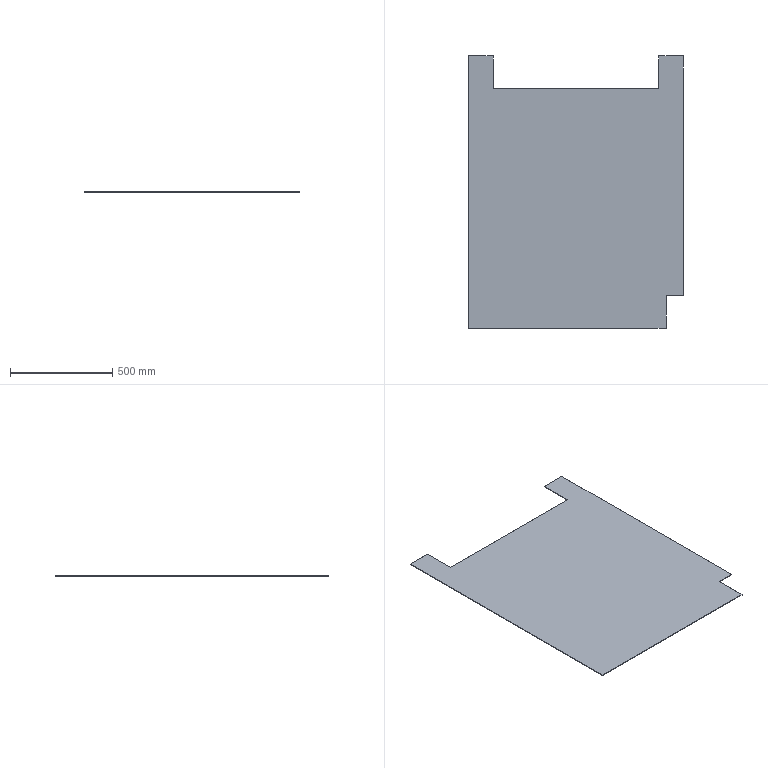Part | STEP file | Electrical cabinet stair checkered plate | 1 solid | 12 faces | box 1050 x 1330 x 3 mm | volume 3760665 mm3 | plane 12
STEP:
#1=CARTESIAN_POINT('',(0.,0.,0.));
#2=DIRECTION('',(0.,0.,1.));
#3=DIRECTION('',(1.,0.,0.));
#4=AXIS2_PLACEMENT_3D('',#1,#2,#3);
#5=CARTESIAN_POINT('',(1215.,107.,0.));
#6=VERTEX_POINT('',#5);
#7=CARTESIAN_POINT('',(1300.,107.,0.));
#8=VERTEX_POINT('',#7);
#9=CARTESIAN_POINT('',(1215.,107.,0.));
#10=DIRECTION('',(1.,0.,0.));
#11=VECTOR('',#10,1.);
#12=LINE('',#9,#11);
#13=CARTESIAN_POINT('',(1215.,107.,3.));
#14=DIRECTION('',(0.,1.,0.));
#15=DIRECTION('',(0.,0.,1.));
#16=AXIS2_PLACEMENT_3D('',#13,#14,#15);
#17=PLANE('',#16);
#18=CARTESIAN_POINT('',(-3.,0.));
#19=DIRECTION('',(0.,1.));
#20=VECTOR('',#19,1.);
#21=LINE('',#18,#20);
#22=(GEOMETRIC_REPRESENTATION_CONTEXT(2)PARAMETRIC_REPRESENTATION_CONTEXT()REPRESENTATION_CONTEXT('',''));
#23=DEFINITIONAL_REPRESENTATION('',(#21),#22);
#24=PCURVE('',#17,#23);
#25=CARTESIAN_POINT('',(0.,0.,0.));
#26=DIRECTION('',(0.,0.,1.));
#27=DIRECTION('',(1.,0.,0.));
#28=AXIS2_PLACEMENT_3D('',#25,#26,#27);
#29=PLANE('',#28);
#30=CARTESIAN_POINT('',(1215.,107.));
#31=DIRECTION('',(1.,0.));
#32=VECTOR('',#31,1.);
#33=LINE('',#30,#32);
#34=(GEOMETRIC_REPRESENTATION_CONTEXT(2)PARAMETRIC_REPRESENTATION_CONTEXT()REPRESENTATION_CONTEXT('',''));
#35=DEFINITIONAL_REPRESENTATION('',(#33),#34);
#36=PCURVE('',#29,#35);
#37=SURFACE_CURVE('',#12,(#24,#36),.PCURVE_S1.);
#38=EDGE_CURVE('',#6,#8,#37,.T.);
#39=ORIENTED_EDGE('',*,*,#38,.T.);
#40=CARTESIAN_POINT('',(1300.,107.,3.));
#41=VERTEX_POINT('',#40);
#42=CARTESIAN_POINT('',(1300.,107.,3.));
#43=DIRECTION('',(0.,0.,-1.));
#44=VECTOR('',#43,1.);
#45=LINE('',#42,#44);
#46=CARTESIAN_POINT('',(0.,85.));
#47=DIRECTION('',(-1.,0.));
#48=VECTOR('',#47,1.);
#49=LINE('',#46,#48);
#50=(GEOMETRIC_REPRESENTATION_CONTEXT(2)PARAMETRIC_REPRESENTATION_CONTEXT()REPRESENTATION_CONTEXT('',''));
#51=DEFINITIONAL_REPRESENTATION('',(#49),#50);
#52=PCURVE('',#17,#51);
#53=CARTESIAN_POINT('',(1300.,107.,3.));
#54=DIRECTION('',(-1.,0.,0.));
#55=DIRECTION('',(0.,-1.,0.));
#56=AXIS2_PLACEMENT_3D('',#53,#54,#55);
#57=PLANE('',#56);
#58=CARTESIAN_POINT('',(0.,0.));
#59=DIRECTION('',(0.,-1.));
#60=VECTOR('',#59,1.);
#61=LINE('',#58,#60);
#62=(GEOMETRIC_REPRESENTATION_CONTEXT(2)PARAMETRIC_REPRESENTATION_CONTEXT()REPRESENTATION_CONTEXT('',''));
#63=DEFINITIONAL_REPRESENTATION('',(#61),#62);
#64=PCURVE('',#57,#63);
#65=SURFACE_CURVE('',#45,(#52,#64),.PCURVE_S1.);
#66=EDGE_CURVE('',#41,#8,#65,.T.);
#67=ORIENTED_EDGE('',*,*,#66,.F.);
#68=CARTESIAN_POINT('',(1215.,107.,3.));
#69=VERTEX_POINT('',#68);
#70=CARTESIAN_POINT('',(1215.,107.,3.));
#71=DIRECTION('',(1.,0.,0.));
#72=VECTOR('',#71,1.);
#73=LINE('',#70,#72);
#74=CARTESIAN_POINT('',(0.,0.));
#75=DIRECTION('',(0.,1.));
#76=VECTOR('',#75,1.);
#77=LINE('',#74,#76);
#78=(GEOMETRIC_REPRESENTATION_CONTEXT(2)PARAMETRIC_REPRESENTATION_CONTEXT()REPRESENTATION_CONTEXT('',''));
#79=DEFINITIONAL_REPRESENTATION('',(#77),#78);
#80=PCURVE('',#17,#79);
#81=CARTESIAN_POINT('',(0.,0.,3.));
#82=DIRECTION('',(0.,0.,1.));
#83=DIRECTION('',(1.,0.,0.));
#84=AXIS2_PLACEMENT_3D('',#81,#82,#83);
#85=PLANE('',#84);
#86=CARTESIAN_POINT('',(1215.,107.));
#87=DIRECTION('',(1.,0.));
#88=VECTOR('',#87,1.);
#89=LINE('',#86,#88);
#90=(GEOMETRIC_REPRESENTATION_CONTEXT(2)PARAMETRIC_REPRESENTATION_CONTEXT()REPRESENTATION_CONTEXT('',''));
#91=DEFINITIONAL_REPRESENTATION('',(#89),#90);
#92=PCURVE('',#85,#91);
#93=SURFACE_CURVE('',#73,(#80,#92),.PCURVE_S1.);
#94=EDGE_CURVE('',#69,#41,#93,.T.);
#95=ORIENTED_EDGE('',*,*,#94,.F.);
#96=CARTESIAN_POINT('',(1215.,107.,3.));
#97=DIRECTION('',(0.,0.,-1.));
#98=VECTOR('',#97,1.);
#99=LINE('',#96,#98);
#100=CARTESIAN_POINT('',(0.,0.));
#101=DIRECTION('',(-1.,0.));
#102=VECTOR('',#101,1.);
#103=LINE('',#100,#102);
#104=(GEOMETRIC_REPRESENTATION_CONTEXT(2)PARAMETRIC_REPRESENTATION_CONTEXT()REPRESENTATION_CONTEXT('',''));
#105=DEFINITIONAL_REPRESENTATION('',(#103),#104);
#106=PCURVE('',#17,#105);
#107=CARTESIAN_POINT('',(1215.,-50.,3.));
#108=DIRECTION('',(-1.,0.,0.));
#109=DIRECTION('',(0.,0.,1.));
#110=AXIS2_PLACEMENT_3D('',#107,#108,#109);
#111=PLANE('',#110);
#112=CARTESIAN_POINT('',(0.,157.));
#113=DIRECTION('',(-1.,0.));
#114=VECTOR('',#113,1.);
#115=LINE('',#112,#114);
#116=(GEOMETRIC_REPRESENTATION_CONTEXT(2)PARAMETRIC_REPRESENTATION_CONTEXT()REPRESENTATION_CONTEXT('',''));
#117=DEFINITIONAL_REPRESENTATION('',(#115),#116);
#118=PCURVE('',#111,#117);
#119=SURFACE_CURVE('',#99,(#106,#118),.PCURVE_S1.);
#120=EDGE_CURVE('',#69,#6,#119,.T.);
#121=ORIENTED_EDGE('',*,*,#120,.T.);
#122=EDGE_LOOP('',(#39,#67,#95,#121));
#123=FACE_BOUND('',#122,.T.);
#124=ADVANCED_FACE('',(#123),#17,.F.);
#125=CARTESIAN_POINT('',(1300.,1280.,0.));
#126=VERTEX_POINT('',#125);
#127=CARTESIAN_POINT('',(1300.,107.,0.));
#128=DIRECTION('',(0.,1.,0.));
#129=VECTOR('',#128,1.);
#130=LINE('',#127,#129);
#131=CARTESIAN_POINT('',(0.,-3.));
#132=DIRECTION('',(-1.,0.));
#133=VECTOR('',#132,1.);
#134=LINE('',#131,#133);
#135=(GEOMETRIC_REPRESENTATION_CONTEXT(2)PARAMETRIC_REPRESENTATION_CONTEXT()REPRESENTATION_CONTEXT('',''));
#136=DEFINITIONAL_REPRESENTATION('',(#134),#135);
#137=PCURVE('',#57,#136);
#138=CARTESIAN_POINT('',(1300.,107.));
#139=DIRECTION('',(0.,1.));
#140=VECTOR('',#139,1.);
#141=LINE('',#138,#140);
#142=(GEOMETRIC_REPRESENTATION_CONTEXT(2)PARAMETRIC_REPRESENTATION_CONTEXT()REPRESENTATION_CONTEXT('',''));
#143=DEFINITIONAL_REPRESENTATION('',(#141),#142);
#144=PCURVE('',#29,#143);
#145=SURFACE_CURVE('',#130,(#137,#144),.PCURVE_S1.);
#146=EDGE_CURVE('',#8,#126,#145,.T.);
#147=ORIENTED_EDGE('',*,*,#146,.T.);
#148=CARTESIAN_POINT('',(1300.,1280.,3.));
#149=VERTEX_POINT('',#148);
#150=CARTESIAN_POINT('',(1300.,1280.,3.));
#151=DIRECTION('',(0.,0.,-1.));
#152=VECTOR('',#151,1.);
#153=LINE('',#150,#152);
#154=CARTESIAN_POINT('',(-1173.,0.));
#155=DIRECTION('',(0.,-1.));
#156=VECTOR('',#155,1.);
#157=LINE('',#154,#156);
#158=(GEOMETRIC_REPRESENTATION_CONTEXT(2)PARAMETRIC_REPRESENTATION_CONTEXT()REPRESENTATION_CONTEXT('',''));
#159=DEFINITIONAL_REPRESENTATION('',(#157),#158);
#160=PCURVE('',#57,#159);
#161=CARTESIAN_POINT('',(1300.,1280.,3.));
#162=DIRECTION('',(0.,-1.,0.));
#163=DIRECTION('',(0.,0.,-1.));
#164=AXIS2_PLACEMENT_3D('',#161,#162,#163);
#165=PLANE('',#164);
#166=CARTESIAN_POINT('',(0.,0.));
#167=DIRECTION('',(1.,0.));
#168=VECTOR('',#167,1.);
#169=LINE('',#166,#168);
#170=(GEOMETRIC_REPRESENTATION_CONTEXT(2)PARAMETRIC_REPRESENTATION_CONTEXT()REPRESENTATION_CONTEXT('',''));
#171=DEFINITIONAL_REPRESENTATION('',(#169),#170);
#172=PCURVE('',#165,#171);
#173=SURFACE_CURVE('',#153,(#160,#172),.PCURVE_S1.);
#174=EDGE_CURVE('',#149,#126,#173,.T.);
#175=ORIENTED_EDGE('',*,*,#174,.F.);
#176=CARTESIAN_POINT('',(1300.,107.,3.));
#177=DIRECTION('',(0.,1.,0.));
#178=VECTOR('',#177,1.);
#179=LINE('',#176,#178);
#180=CARTESIAN_POINT('',(0.,0.));
#181=DIRECTION('',(-1.,0.));
#182=VECTOR('',#181,1.);
#183=LINE('',#180,#182);
#184=(GEOMETRIC_REPRESENTATION_CONTEXT(2)PARAMETRIC_REPRESENTATION_CONTEXT()REPRESENTATION_CONTEXT('',''));
#185=DEFINITIONAL_REPRESENTATION('',(#183),#184);
#186=PCURVE('',#57,#185);
#187=CARTESIAN_POINT('',(1300.,107.));
#188=DIRECTION('',(0.,1.));
#189=VECTOR('',#188,1.);
#190=LINE('',#187,#189);
#191=(GEOMETRIC_REPRESENTATION_CONTEXT(2)PARAMETRIC_REPRESENTATION_CONTEXT()REPRESENTATION_CONTEXT('',''));
#192=DEFINITIONAL_REPRESENTATION('',(#190),#191);
#193=PCURVE('',#85,#192);
#194=SURFACE_CURVE('',#179,(#186,#193),.PCURVE_S1.);
#195=EDGE_CURVE('',#41,#149,#194,.T.);
#196=ORIENTED_EDGE('',*,*,#195,.F.);
#197=ORIENTED_EDGE('',*,*,#66,.T.);
#198=EDGE_LOOP('',(#147,#175,#196,#197));
#199=FACE_BOUND('',#198,.T.);
#200=ADVANCED_FACE('',(#199),#57,.F.);
#201=CARTESIAN_POINT('',(1180.,1280.,0.));
#202=VERTEX_POINT('',#201);
#203=CARTESIAN_POINT('',(1300.,1280.,0.));
#204=DIRECTION('',(-1.,0.,0.));
#205=VECTOR('',#204,1.);
#206=LINE('',#203,#205);
#207=CARTESIAN_POINT('',(3.,0.));
#208=DIRECTION('',(0.,-1.));
#209=VECTOR('',#208,1.);
#210=LINE('',#207,#209);
#211=(GEOMETRIC_REPRESENTATION_CONTEXT(2)PARAMETRIC_REPRESENTATION_CONTEXT()REPRESENTATION_CONTEXT('',''));
#212=DEFINITIONAL_REPRESENTATION('',(#210),#211);
#213=PCURVE('',#165,#212);
#214=CARTESIAN_POINT('',(1300.,1280.));
#215=DIRECTION('',(-1.,0.));
#216=VECTOR('',#215,1.);
#217=LINE('',#214,#216);
#218=(GEOMETRIC_REPRESENTATION_CONTEXT(2)PARAMETRIC_REPRESENTATION_CONTEXT()REPRESENTATION_CONTEXT('',''));
#219=DEFINITIONAL_REPRESENTATION('',(#217),#218);
#220=PCURVE('',#29,#219);
#221=SURFACE_CURVE('',#206,(#213,#220),.PCURVE_S1.);
#222=EDGE_CURVE('',#126,#202,#221,.T.);
#223=ORIENTED_EDGE('',*,*,#222,.T.);
#224=CARTESIAN_POINT('',(1180.,1280.,3.));
#225=VERTEX_POINT('',#224);
#226=CARTESIAN_POINT('',(1180.,1280.,3.));
#227=DIRECTION('',(0.,0.,-1.));
#228=VECTOR('',#227,1.);
#229=LINE('',#226,#228);
#230=CARTESIAN_POINT('',(0.,-120.));
#231=DIRECTION('',(1.,0.));
#232=VECTOR('',#231,1.);
#233=LINE('',#230,#232);
#234=(GEOMETRIC_REPRESENTATION_CONTEXT(2)PARAMETRIC_REPRESENTATION_CONTEXT()REPRESENTATION_CONTEXT('',''));
#235=DEFINITIONAL_REPRESENTATION('',(#233),#234);
#236=PCURVE('',#165,#235);
#237=CARTESIAN_POINT('',(1180.,1120.,3.));
#238=DIRECTION('',(1.,0.,0.));
#239=DIRECTION('',(0.,0.,-1.));
#240=AXIS2_PLACEMENT_3D('',#237,#238,#239);
#241=PLANE('',#240);
#242=CARTESIAN_POINT('',(0.,160.));
#243=DIRECTION('',(1.,0.));
#244=VECTOR('',#243,1.);
#245=LINE('',#242,#244);
#246=(GEOMETRIC_REPRESENTATION_CONTEXT(2)PARAMETRIC_REPRESENTATION_CONTEXT()REPRESENTATION_CONTEXT('',''));
#247=DEFINITIONAL_REPRESENTATION('',(#245),#246);
#248=PCURVE('',#241,#247);
#249=SURFACE_CURVE('',#229,(#236,#248),.PCURVE_S1.);
#250=EDGE_CURVE('',#225,#202,#249,.T.);
#251=ORIENTED_EDGE('',*,*,#250,.F.);
#252=CARTESIAN_POINT('',(1300.,1280.,3.));
#253=DIRECTION('',(-1.,0.,0.));
#254=VECTOR('',#253,1.);
#255=LINE('',#252,#254);
#256=CARTESIAN_POINT('',(0.,0.));
#257=DIRECTION('',(0.,-1.));
#258=VECTOR('',#257,1.);
#259=LINE('',#256,#258);
#260=(GEOMETRIC_REPRESENTATION_CONTEXT(2)PARAMETRIC_REPRESENTATION_CONTEXT()REPRESENTATION_CONTEXT('',''));
#261=DEFINITIONAL_REPRESENTATION('',(#259),#260);
#262=PCURVE('',#165,#261);
#263=CARTESIAN_POINT('',(1300.,1280.));
#264=DIRECTION('',(-1.,0.));
#265=VECTOR('',#264,1.);
#266=LINE('',#263,#265);
#267=(GEOMETRIC_REPRESENTATION_CONTEXT(2)PARAMETRIC_REPRESENTATION_CONTEXT()REPRESENTATION_CONTEXT('',''));
#268=DEFINITIONAL_REPRESENTATION('',(#266),#267);
#269=PCURVE('',#85,#268);
#270=SURFACE_CURVE('',#255,(#262,#269),.PCURVE_S1.);
#271=EDGE_CURVE('',#149,#225,#270,.T.);
#272=ORIENTED_EDGE('',*,*,#271,.F.);
#273=ORIENTED_EDGE('',*,*,#174,.T.);
#274=EDGE_LOOP('',(#223,#251,#272,#273));
#275=FACE_BOUND('',#274,.T.);
#276=ADVANCED_FACE('',(#275),#165,.F.);
#277=CARTESIAN_POINT('',(1180.,1120.,0.));
#278=VERTEX_POINT('',#277);
#279=CARTESIAN_POINT('',(1180.,1120.,0.));
#280=DIRECTION('',(0.,-1.,0.));
#281=VECTOR('',#280,1.);
#282=LINE('',#279,#281);
#283=CARTESIAN_POINT('',(3.,0.));
#284=DIRECTION('',(0.,-1.));
#285=VECTOR('',#284,1.);
#286=LINE('',#283,#285);
#287=(GEOMETRIC_REPRESENTATION_CONTEXT(2)PARAMETRIC_REPRESENTATION_CONTEXT()REPRESENTATION_CONTEXT('',''));
#288=DEFINITIONAL_REPRESENTATION('',(#286),#287);
#289=PCURVE('',#241,#288);
#290=CARTESIAN_POINT('',(1180.,1120.));
#291=DIRECTION('',(0.,-1.));
#292=VECTOR('',#291,1.);
#293=LINE('',#290,#292);
#294=(GEOMETRIC_REPRESENTATION_CONTEXT(2)PARAMETRIC_REPRESENTATION_CONTEXT()REPRESENTATION_CONTEXT('',''));
#295=DEFINITIONAL_REPRESENTATION('',(#293),#294);
#296=PCURVE('',#29,#295);
#297=SURFACE_CURVE('',#282,(#289,#296),.PCURVE_S1.);
#298=EDGE_CURVE('',#202,#278,#297,.T.);
#299=ORIENTED_EDGE('',*,*,#298,.T.);
#300=CARTESIAN_POINT('',(1180.,1120.,3.));
#301=VERTEX_POINT('',#300);
#302=CARTESIAN_POINT('',(1180.,1120.,3.));
#303=DIRECTION('',(0.,0.,-1.));
#304=VECTOR('',#303,1.);
#305=LINE('',#302,#304);
#306=CARTESIAN_POINT('',(0.,0.));
#307=DIRECTION('',(1.,0.));
#308=VECTOR('',#307,1.);
#309=LINE('',#306,#308);
#310=(GEOMETRIC_REPRESENTATION_CONTEXT(2)PARAMETRIC_REPRESENTATION_CONTEXT()REPRESENTATION_CONTEXT('',''));
#311=DEFINITIONAL_REPRESENTATION('',(#309),#310);
#312=PCURVE('',#241,#311);
#313=CARTESIAN_POINT('',(370.,1120.,3.));
#314=DIRECTION('',(0.,-1.,0.));
#315=DIRECTION('',(0.,0.,-1.));
#316=AXIS2_PLACEMENT_3D('',#313,#314,#315);
#317=PLANE('',#316);
#318=CARTESIAN_POINT('',(0.,810.));
#319=DIRECTION('',(1.,0.));
#320=VECTOR('',#319,1.);
#321=LINE('',#318,#320);
#322=(GEOMETRIC_REPRESENTATION_CONTEXT(2)PARAMETRIC_REPRESENTATION_CONTEXT()REPRESENTATION_CONTEXT('',''));
#323=DEFINITIONAL_REPRESENTATION('',(#321),#322);
#324=PCURVE('',#317,#323);
#325=SURFACE_CURVE('',#305,(#312,#324),.PCURVE_S1.);
#326=EDGE_CURVE('',#301,#278,#325,.T.);
#327=ORIENTED_EDGE('',*,*,#326,.F.);
#328=CARTESIAN_POINT('',(1180.,1120.,3.));
#329=DIRECTION('',(0.,-1.,0.));
#330=VECTOR('',#329,1.);
#331=LINE('',#328,#330);
#332=CARTESIAN_POINT('',(0.,0.));
#333=DIRECTION('',(0.,-1.));
#334=VECTOR('',#333,1.);
#335=LINE('',#332,#334);
#336=(GEOMETRIC_REPRESENTATION_CONTEXT(2)PARAMETRIC_REPRESENTATION_CONTEXT()REPRESENTATION_CONTEXT('',''));
#337=DEFINITIONAL_REPRESENTATION('',(#335),#336);
#338=PCURVE('',#241,#337);
#339=CARTESIAN_POINT('',(1180.,1120.));
#340=DIRECTION('',(0.,-1.));
#341=VECTOR('',#340,1.);
#342=LINE('',#339,#341);
#343=(GEOMETRIC_REPRESENTATION_CONTEXT(2)PARAMETRIC_REPRESENTATION_CONTEXT()REPRESENTATION_CONTEXT('',''));
#344=DEFINITIONAL_REPRESENTATION('',(#342),#343);
#345=PCURVE('',#85,#344);
#346=SURFACE_CURVE('',#331,(#338,#345),.PCURVE_S1.);
#347=EDGE_CURVE('',#225,#301,#346,.T.);
#348=ORIENTED_EDGE('',*,*,#347,.F.);
#349=ORIENTED_EDGE('',*,*,#250,.T.);
#350=EDGE_LOOP('',(#299,#327,#348,#349));
#351=FACE_BOUND('',#350,.T.);
#352=ADVANCED_FACE('',(#351),#241,.F.);
#353=CARTESIAN_POINT('',(370.,1120.,0.));
#354=VERTEX_POINT('',#353);
#355=CARTESIAN_POINT('',(370.,1120.,0.));
#356=DIRECTION('',(-1.,0.,0.));
#357=VECTOR('',#356,1.);
#358=LINE('',#355,#357);
#359=CARTESIAN_POINT('',(3.,0.));
#360=DIRECTION('',(0.,-1.));
#361=VECTOR('',#360,1.);
#362=LINE('',#359,#361);
#363=(GEOMETRIC_REPRESENTATION_CONTEXT(2)PARAMETRIC_REPRESENTATION_CONTEXT()REPRESENTATION_CONTEXT('',''));
#364=DEFINITIONAL_REPRESENTATION('',(#362),#363);
#365=PCURVE('',#317,#364);
#366=CARTESIAN_POINT('',(370.,1120.));
#367=DIRECTION('',(-1.,0.));
#368=VECTOR('',#367,1.);
#369=LINE('',#366,#368);
#370=(GEOMETRIC_REPRESENTATION_CONTEXT(2)PARAMETRIC_REPRESENTATION_CONTEXT()REPRESENTATION_CONTEXT('',''));
#371=DEFINITIONAL_REPRESENTATION('',(#369),#370);
#372=PCURVE('',#29,#371);
#373=SURFACE_CURVE('',#358,(#365,#372),.PCURVE_S1.);
#374=EDGE_CURVE('',#278,#354,#373,.T.);
#375=ORIENTED_EDGE('',*,*,#374,.T.);
#376=CARTESIAN_POINT('',(370.,1120.,3.));
#377=VERTEX_POINT('',#376);
#378=CARTESIAN_POINT('',(370.,1120.,3.));
#379=DIRECTION('',(0.,0.,-1.));
#380=VECTOR('',#379,1.);
#381=LINE('',#378,#380);
#382=CARTESIAN_POINT('',(0.,0.));
#383=DIRECTION('',(1.,0.));
#384=VECTOR('',#383,1.);
#385=LINE('',#382,#384);
#386=(GEOMETRIC_REPRESENTATION_CONTEXT(2)PARAMETRIC_REPRESENTATION_CONTEXT()REPRESENTATION_CONTEXT('',''));
#387=DEFINITIONAL_REPRESENTATION('',(#385),#386);
#388=PCURVE('',#317,#387);
#389=CARTESIAN_POINT('',(370.,1280.,3.));
#390=DIRECTION('',(-1.,0.,0.));
#391=DIRECTION('',(0.,0.,1.));
#392=AXIS2_PLACEMENT_3D('',#389,#390,#391);
#393=PLANE('',#392);
#394=CARTESIAN_POINT('',(0.,-160.));
#395=DIRECTION('',(-1.,0.));
#396=VECTOR('',#395,1.);
#397=LINE('',#394,#396);
#398=(GEOMETRIC_REPRESENTATION_CONTEXT(2)PARAMETRIC_REPRESENTATION_CONTEXT()REPRESENTATION_CONTEXT('',''));
#399=DEFINITIONAL_REPRESENTATION('',(#397),#398);
#400=PCURVE('',#393,#399);
#401=SURFACE_CURVE('',#381,(#388,#400),.PCURVE_S1.);
#402=EDGE_CURVE('',#377,#354,#401,.T.);
#403=ORIENTED_EDGE('',*,*,#402,.F.);
#404=CARTESIAN_POINT('',(370.,1120.,3.));
#405=DIRECTION('',(-1.,0.,0.));
#406=VECTOR('',#405,1.);
#407=LINE('',#404,#406);
#408=CARTESIAN_POINT('',(0.,0.));
#409=DIRECTION('',(0.,-1.));
#410=VECTOR('',#409,1.);
#411=LINE('',#408,#410);
#412=(GEOMETRIC_REPRESENTATION_CONTEXT(2)PARAMETRIC_REPRESENTATION_CONTEXT()REPRESENTATION_CONTEXT('',''));
#413=DEFINITIONAL_REPRESENTATION('',(#411),#412);
#414=PCURVE('',#317,#413);
#415=CARTESIAN_POINT('',(370.,1120.));
#416=DIRECTION('',(-1.,0.));
#417=VECTOR('',#416,1.);
#418=LINE('',#415,#417);
#419=(GEOMETRIC_REPRESENTATION_CONTEXT(2)PARAMETRIC_REPRESENTATION_CONTEXT()REPRESENTATION_CONTEXT('',''));
#420=DEFINITIONAL_REPRESENTATION('',(#418),#419);
#421=PCURVE('',#85,#420);
#422=SURFACE_CURVE('',#407,(#414,#421),.PCURVE_S1.);
#423=EDGE_CURVE('',#301,#377,#422,.T.);
#424=ORIENTED_EDGE('',*,*,#423,.F.);
#425=ORIENTED_EDGE('',*,*,#326,.T.);
#426=EDGE_LOOP('',(#375,#403,#424,#425));
#427=FACE_BOUND('',#426,.T.);
#428=ADVANCED_FACE('',(#427),#317,.F.);
#429=CARTESIAN_POINT('',(370.,1280.,0.));
#430=VERTEX_POINT('',#429);
#431=CARTESIAN_POINT('',(370.,1280.,0.));
#432=DIRECTION('',(0.,1.,0.));
#433=VECTOR('',#432,1.);
#434=LINE('',#431,#433);
#435=CARTESIAN_POINT('',(-3.,0.));
#436=DIRECTION('',(0.,1.));
#437=VECTOR('',#436,1.);
#438=LINE('',#435,#437);
#439=(GEOMETRIC_REPRESENTATION_CONTEXT(2)PARAMETRIC_REPRESENTATION_CONTEXT()REPRESENTATION_CONTEXT('',''));
#440=DEFINITIONAL_REPRESENTATION('',(#438),#439);
#441=PCURVE('',#393,#440);
#442=CARTESIAN_POINT('',(370.,1280.));
#443=DIRECTION('',(0.,1.));
#444=VECTOR('',#443,1.);
#445=LINE('',#442,#444);
#446=(GEOMETRIC_REPRESENTATION_CONTEXT(2)PARAMETRIC_REPRESENTATION_CONTEXT()REPRESENTATION_CONTEXT('',''));
#447=DEFINITIONAL_REPRESENTATION('',(#445),#446);
#448=PCURVE('',#29,#447);
#449=SURFACE_CURVE('',#434,(#441,#448),.PCURVE_S1.);
#450=EDGE_CURVE('',#354,#430,#449,.T.);
#451=ORIENTED_EDGE('',*,*,#450,.T.);
#452=CARTESIAN_POINT('',(370.,1280.,3.));
#453=VERTEX_POINT('',#452);
#454=CARTESIAN_POINT('',(370.,1280.,3.));
#455=DIRECTION('',(0.,0.,-1.));
#456=VECTOR('',#455,1.);
#457=LINE('',#454,#456);
#458=CARTESIAN_POINT('',(0.,0.));
#459=DIRECTION('',(-1.,0.));
#460=VECTOR('',#459,1.);
#461=LINE('',#458,#460);
#462=(GEOMETRIC_REPRESENTATION_CONTEXT(2)PARAMETRIC_REPRESENTATION_CONTEXT()REPRESENTATION_CONTEXT('',''));
#463=DEFINITIONAL_REPRESENTATION('',(#461),#462);
#464=PCURVE('',#393,#463);
#465=CARTESIAN_POINT('',(370.,1280.,3.));
#466=DIRECTION('',(0.,-1.,0.));
#467=DIRECTION('',(0.,0.,-1.));
#468=AXIS2_PLACEMENT_3D('',#465,#466,#467);
#469=PLANE('',#468);
#470=CARTESIAN_POINT('',(0.,0.));
#471=DIRECTION('',(1.,0.));
#472=VECTOR('',#471,1.);
#473=LINE('',#470,#472);
#474=(GEOMETRIC_REPRESENTATION_CONTEXT(2)PARAMETRIC_REPRESENTATION_CONTEXT()REPRESENTATION_CONTEXT('',''));
#475=DEFINITIONAL_REPRESENTATION('',(#473),#474);
#476=PCURVE('',#469,#475);
#477=SURFACE_CURVE('',#457,(#464,#476),.PCURVE_S1.);
#478=EDGE_CURVE('',#453,#430,#477,.T.);
#479=ORIENTED_EDGE('',*,*,#478,.F.);
#480=CARTESIAN_POINT('',(370.,1280.,3.));
#481=DIRECTION('',(0.,1.,0.));
#482=VECTOR('',#481,1.);
#483=LINE('',#480,#482);
#484=CARTESIAN_POINT('',(0.,0.));
#485=DIRECTION('',(0.,1.));
#486=VECTOR('',#485,1.);
#487=LINE('',#484,#486);
#488=(GEOMETRIC_REPRESENTATION_CONTEXT(2)PARAMETRIC_REPRESENTATION_CONTEXT()REPRESENTATION_CONTEXT('',''));
#489=DEFINITIONAL_REPRESENTATION('',(#487),#488);
#490=PCURVE('',#393,#489);
#491=CARTESIAN_POINT('',(370.,1280.));
#492=DIRECTION('',(0.,1.));
#493=VECTOR('',#492,1.);
#494=LINE('',#491,#493);
#495=(GEOMETRIC_REPRESENTATION_CONTEXT(2)PARAMETRIC_REPRESENTATION_CONTEXT()REPRESENTATION_CONTEXT('',''));
#496=DEFINITIONAL_REPRESENTATION('',(#494),#495);
#497=PCURVE('',#85,#496);
#498=SURFACE_CURVE('',#483,(#490,#497),.PCURVE_S1.);
#499=EDGE_CURVE('',#377,#453,#498,.T.);
#500=ORIENTED_EDGE('',*,*,#499,.F.);
#501=ORIENTED_EDGE('',*,*,#402,.T.);
#502=EDGE_LOOP('',(#451,#479,#500,#501));
#503=FACE_BOUND('',#502,.T.);
#504=ADVANCED_FACE('',(#503),#393,.F.);
#505=CARTESIAN_POINT('',(250.,1280.,0.));
#506=VERTEX_POINT('',#505);
#507=CARTESIAN_POINT('',(370.,1280.,0.));
#508=DIRECTION('',(-1.,0.,0.));
#509=VECTOR('',#508,1.);
#510=LINE('',#507,#509);
#511=CARTESIAN_POINT('',(3.,0.));
#512=DIRECTION('',(0.,-1.));
#513=VECTOR('',#512,1.);
#514=LINE('',#511,#513);
#515=(GEOMETRIC_REPRESENTATION_CONTEXT(2)PARAMETRIC_REPRESENTATION_CONTEXT()REPRESENTATION_CONTEXT('',''));
#516=DEFINITIONAL_REPRESENTATION('',(#514),#515);
#517=PCURVE('',#469,#516);
#518=CARTESIAN_POINT('',(370.,1280.));
#519=DIRECTION('',(-1.,0.));
#520=VECTOR('',#519,1.);
#521=LINE('',#518,#520);
#522=(GEOMETRIC_REPRESENTATION_CONTEXT(2)PARAMETRIC_REPRESENTATION_CONTEXT()REPRESENTATION_CONTEXT('',''));
#523=DEFINITIONAL_REPRESENTATION('',(#521),#522);
#524=PCURVE('',#29,#523);
#525=SURFACE_CURVE('',#510,(#517,#524),.PCURVE_S1.);
#526=EDGE_CURVE('',#430,#506,#525,.T.);
#527=ORIENTED_EDGE('',*,*,#526,.T.);
#528=CARTESIAN_POINT('',(250.,1280.,3.));
#529=VERTEX_POINT('',#528);
#530=CARTESIAN_POINT('',(250.,1280.,3.));
#531=DIRECTION('',(0.,0.,-1.));
#532=VECTOR('',#531,1.);
#533=LINE('',#530,#532);
#534=CARTESIAN_POINT('',(0.,-120.));
#535=DIRECTION('',(1.,0.));
#536=VECTOR('',#535,1.);
#537=LINE('',#534,#536);
#538=(GEOMETRIC_REPRESENTATION_CONTEXT(2)PARAMETRIC_REPRESENTATION_CONTEXT()REPRESENTATION_CONTEXT('',''));
#539=DEFINITIONAL_REPRESENTATION('',(#537),#538);
#540=PCURVE('',#469,#539);
#541=CARTESIAN_POINT('',(250.,1280.,3.));
#542=DIRECTION('',(1.,0.,0.));
#543=DIRECTION('',(0.,1.,0.));
#544=AXIS2_PLACEMENT_3D('',#541,#542,#543);
#545=PLANE('',#544);
#546=CARTESIAN_POINT('',(0.,0.));
#547=DIRECTION('',(0.,-1.));
#548=VECTOR('',#547,1.);
#549=LINE('',#546,#548);
#550=(GEOMETRIC_REPRESENTATION_CONTEXT(2)PARAMETRIC_REPRESENTATION_CONTEXT()REPRESENTATION_CONTEXT('',''));
#551=DEFINITIONAL_REPRESENTATION('',(#549),#550);
#552=PCURVE('',#545,#551);
#553=SURFACE_CURVE('',#533,(#540,#552),.PCURVE_S1.);
#554=EDGE_CURVE('',#529,#506,#553,.T.);
#555=ORIENTED_EDGE('',*,*,#554,.F.);
#556=CARTESIAN_POINT('',(370.,1280.,3.));
#557=DIRECTION('',(-1.,0.,0.));
#558=VECTOR('',#557,1.);
#559=LINE('',#556,#558);
#560=CARTESIAN_POINT('',(0.,0.));
#561=DIRECTION('',(0.,-1.));
#562=VECTOR('',#561,1.);
#563=LINE('',#560,#562);
#564=(GEOMETRIC_REPRESENTATION_CONTEXT(2)PARAMETRIC_REPRESENTATION_CONTEXT()REPRESENTATION_CONTEXT('',''));
#565=DEFINITIONAL_REPRESENTATION('',(#563),#564);
#566=PCURVE('',#469,#565);
#567=CARTESIAN_POINT('',(370.,1280.));
#568=DIRECTION('',(-1.,0.));
#569=VECTOR('',#568,1.);
#570=LINE('',#567,#569);
#571=(GEOMETRIC_REPRESENTATION_CONTEXT(2)PARAMETRIC_REPRESENTATION_CONTEXT()REPRESENTATION_CONTEXT('',''));
#572=DEFINITIONAL_REPRESENTATION('',(#570),#571);
#573=PCURVE('',#85,#572);
#574=SURFACE_CURVE('',#559,(#566,#573),.PCURVE_S1.);
#575=EDGE_CURVE('',#453,#529,#574,.T.);
#576=ORIENTED_EDGE('',*,*,#575,.F.);
#577=ORIENTED_EDGE('',*,*,#478,.T.);
#578=EDGE_LOOP('',(#527,#555,#576,#577));
#579=FACE_BOUND('',#578,.T.);
#580=ADVANCED_FACE('',(#579),#469,.F.);
#581=CARTESIAN_POINT('',(250.,-50.,0.));
#582=VERTEX_POINT('',#581);
#583=CARTESIAN_POINT('',(250.,1280.,0.));
#584=DIRECTION('',(0.,-1.,0.));
#585=VECTOR('',#584,1.);
#586=LINE('',#583,#585);
#587=CARTESIAN_POINT('',(0.,-3.));
#588=DIRECTION('',(-1.,0.));
#589=VECTOR('',#588,1.);
#590=LINE('',#587,#589);
#591=(GEOMETRIC_REPRESENTATION_CONTEXT(2)PARAMETRIC_REPRESENTATION_CONTEXT()REPRESENTATION_CONTEXT('',''));
#592=DEFINITIONAL_REPRESENTATION('',(#590),#591);
#593=PCURVE('',#545,#592);
#594=CARTESIAN_POINT('',(250.,1280.));
#595=DIRECTION('',(0.,-1.));
#596=VECTOR('',#595,1.);
#597=LINE('',#594,#596);
#598=(GEOMETRIC_REPRESENTATION_CONTEXT(2)PARAMETRIC_REPRESENTATION_CONTEXT()REPRESENTATION_CONTEXT('',''));
#599=DEFINITIONAL_REPRESENTATION('',(#597),#598);
#600=PCURVE('',#29,#599);
#601=SURFACE_CURVE('',#586,(#593,#600),.PCURVE_S1.);
#602=EDGE_CURVE('',#506,#582,#601,.T.);
#603=ORIENTED_EDGE('',*,*,#602,.T.);
#604=CARTESIAN_POINT('',(250.,-50.,3.));
#605=VERTEX_POINT('',#604);
#606=CARTESIAN_POINT('',(250.,-50.,3.));
#607=DIRECTION('',(0.,0.,-1.));
#608=VECTOR('',#607,1.);
#609=LINE('',#606,#608);
#610=CARTESIAN_POINT('',(-1330.,0.));
#611=DIRECTION('',(0.,-1.));
#612=VECTOR('',#611,1.);
#613=LINE('',#610,#612);
#614=(GEOMETRIC_REPRESENTATION_CONTEXT(2)PARAMETRIC_REPRESENTATION_CONTEXT()REPRESENTATION_CONTEXT('',''));
#615=DEFINITIONAL_REPRESENTATION('',(#613),#614);
#616=PCURVE('',#545,#615);
#617=CARTESIAN_POINT('',(250.,-50.,3.));
#618=DIRECTION('',(0.,1.,0.));
#619=DIRECTION('',(-1.,0.,0.));
#620=AXIS2_PLACEMENT_3D('',#617,#618,#619);
#621=PLANE('',#620);
#622=CARTESIAN_POINT('',(0.,0.));
#623=DIRECTION('',(0.,-1.));
#624=VECTOR('',#623,1.);
#625=LINE('',#622,#624);
#626=(GEOMETRIC_REPRESENTATION_CONTEXT(2)PARAMETRIC_REPRESENTATION_CONTEXT()REPRESENTATION_CONTEXT('',''));
#627=DEFINITIONAL_REPRESENTATION('',(#625),#626);
#628=PCURVE('',#621,#627);
#629=SURFACE_CURVE('',#609,(#616,#628),.PCURVE_S1.);
#630=EDGE_CURVE('',#605,#582,#629,.T.);
#631=ORIENTED_EDGE('',*,*,#630,.F.);
#632=CARTESIAN_POINT('',(250.,1280.,3.));
#633=DIRECTION('',(0.,-1.,0.));
#634=VECTOR('',#633,1.);
#635=LINE('',#632,#634);
#636=CARTESIAN_POINT('',(0.,0.));
#637=DIRECTION('',(-1.,0.));
#638=VECTOR('',#637,1.);
#639=LINE('',#636,#638);
#640=(GEOMETRIC_REPRESENTATION_CONTEXT(2)PARAMETRIC_REPRESENTATION_CONTEXT()REPRESENTATION_CONTEXT('',''));
#641=DEFINITIONAL_REPRESENTATION('',(#639),#640);
#642=PCURVE('',#545,#641);
#643=CARTESIAN_POINT('',(250.,1280.));
#644=DIRECTION('',(0.,-1.));
#645=VECTOR('',#644,1.);
#646=LINE('',#643,#645);
#647=(GEOMETRIC_REPRESENTATION_CONTEXT(2)PARAMETRIC_REPRESENTATION_CONTEXT()REPRESENTATION_CONTEXT('',''));
#648=DEFINITIONAL_REPRESENTATION('',(#646),#647);
#649=PCURVE('',#85,#648);
#650=SURFACE_CURVE('',#635,(#642,#649),.PCURVE_S1.);
#651=EDGE_CURVE('',#529,#605,#650,.T.);
#652=ORIENTED_EDGE('',*,*,#651,.F.);
#653=ORIENTED_EDGE('',*,*,#554,.T.);
#654=EDGE_LOOP('',(#603,#631,#652,#653));
#655=FACE_BOUND('',#654,.T.);
#656=ADVANCED_FACE('',(#655),#545,.F.);
#657=CARTESIAN_POINT('',(1215.,-50.,0.));
#658=VERTEX_POINT('',#657);
#659=CARTESIAN_POINT('',(250.,-50.,0.));
#660=DIRECTION('',(1.,0.,0.));
#661=VECTOR('',#660,1.);
#662=LINE('',#659,#661);
#663=CARTESIAN_POINT('',(0.,-3.));
#664=DIRECTION('',(-1.,0.));
#665=VECTOR('',#664,1.);
#666=LINE('',#663,#665);
#667=(GEOMETRIC_REPRESENTATION_CONTEXT(2)PARAMETRIC_REPRESENTATION_CONTEXT()REPRESENTATION_CONTEXT('',''));
#668=DEFINITIONAL_REPRESENTATION('',(#666),#667);
#669=PCURVE('',#621,#668);
#670=CARTESIAN_POINT('',(250.,-50.));
#671=DIRECTION('',(1.,0.));
#672=VECTOR('',#671,1.);
#673=LINE('',#670,#672);
#674=(GEOMETRIC_REPRESENTATION_CONTEXT(2)PARAMETRIC_REPRESENTATION_CONTEXT()REPRESENTATION_CONTEXT('',''));
#675=DEFINITIONAL_REPRESENTATION('',(#673),#674);
#676=PCURVE('',#29,#675);
#677=SURFACE_CURVE('',#662,(#669,#676),.PCURVE_S1.);
#678=EDGE_CURVE('',#582,#658,#677,.T.);
#679=ORIENTED_EDGE('',*,*,#678,.T.);
#680=CARTESIAN_POINT('',(1215.,-50.,3.));
#681=VERTEX_POINT('',#680);
#682=CARTESIAN_POINT('',(1215.,-50.,3.));
#683=DIRECTION('',(0.,0.,-1.));
#684=VECTOR('',#683,1.);
#685=LINE('',#682,#684);
#686=CARTESIAN_POINT('',(-965.,0.));
#687=DIRECTION('',(0.,-1.));
#688=VECTOR('',#687,1.);
#689=LINE('',#686,#688);
#690=(GEOMETRIC_REPRESENTATION_CONTEXT(2)PARAMETRIC_REPRESENTATION_CONTEXT()REPRESENTATION_CONTEXT('',''));
#691=DEFINITIONAL_REPRESENTATION('',(#689),#690);
#692=PCURVE('',#621,#691);
#693=CARTESIAN_POINT('',(0.,0.));
#694=DIRECTION('',(-1.,0.));
#695=VECTOR('',#694,1.);
#696=LINE('',#693,#695);
#697=(GEOMETRIC_REPRESENTATION_CONTEXT(2)PARAMETRIC_REPRESENTATION_CONTEXT()REPRESENTATION_CONTEXT('',''));
#698=DEFINITIONAL_REPRESENTATION('',(#696),#697);
#699=PCURVE('',#111,#698);
#700=SURFACE_CURVE('',#685,(#692,#699),.PCURVE_S1.);
#701=EDGE_CURVE('',#681,#658,#700,.T.);
#702=ORIENTED_EDGE('',*,*,#701,.F.);
#703=CARTESIAN_POINT('',(250.,-50.,3.));
#704=DIRECTION('',(1.,0.,0.));
#705=VECTOR('',#704,1.);
#706=LINE('',#703,#705);
#707=CARTESIAN_POINT('',(0.,0.));
#708=DIRECTION('',(-1.,0.));
#709=VECTOR('',#708,1.);
#710=LINE('',#707,#709);
#711=(GEOMETRIC_REPRESENTATION_CONTEXT(2)PARAMETRIC_REPRESENTATION_CONTEXT()REPRESENTATION_CONTEXT('',''));
#712=DEFINITIONAL_REPRESENTATION('',(#710),#711);
#713=PCURVE('',#621,#712);
#714=CARTESIAN_POINT('',(250.,-50.));
#715=DIRECTION('',(1.,0.));
#716=VECTOR('',#715,1.);
#717=LINE('',#714,#716);
#718=(GEOMETRIC_REPRESENTATION_CONTEXT(2)PARAMETRIC_REPRESENTATION_CONTEXT()REPRESENTATION_CONTEXT('',''));
#719=DEFINITIONAL_REPRESENTATION('',(#717),#718);
#720=PCURVE('',#85,#719);
#721=SURFACE_CURVE('',#706,(#713,#720),.PCURVE_S1.);
#722=EDGE_CURVE('',#605,#681,#721,.T.);
#723=ORIENTED_EDGE('',*,*,#722,.F.);
#724=ORIENTED_EDGE('',*,*,#630,.T.);
#725=EDGE_LOOP('',(#679,#702,#723,#724));
#726=FACE_BOUND('',#725,.T.);
#727=ADVANCED_FACE('',(#726),#621,.F.);
#728=CARTESIAN_POINT('',(1215.,-50.,0.));
#729=DIRECTION('',(0.,1.,0.));
#730=VECTOR('',#729,1.);
#731=LINE('',#728,#730);
#732=CARTESIAN_POINT('',(-3.,0.));
#733=DIRECTION('',(0.,1.));
#734=VECTOR('',#733,1.);
#735=LINE('',#732,#734);
#736=(GEOMETRIC_REPRESENTATION_CONTEXT(2)PARAMETRIC_REPRESENTATION_CONTEXT()REPRESENTATION_CONTEXT('',''));
#737=DEFINITIONAL_REPRESENTATION('',(#735),#736);
#738=PCURVE('',#111,#737);
#739=CARTESIAN_POINT('',(1215.,-50.));
#740=DIRECTION('',(0.,1.));
#741=VECTOR('',#740,1.);
#742=LINE('',#739,#741);
#743=(GEOMETRIC_REPRESENTATION_CONTEXT(2)PARAMETRIC_REPRESENTATION_CONTEXT()REPRESENTATION_CONTEXT('',''));
#744=DEFINITIONAL_REPRESENTATION('',(#742),#743);
#745=PCURVE('',#29,#744);
#746=SURFACE_CURVE('',#731,(#738,#745),.PCURVE_S1.);
#747=EDGE_CURVE('',#658,#6,#746,.T.);
#748=ORIENTED_EDGE('',*,*,#747,.T.);
#749=ORIENTED_EDGE('',*,*,#120,.F.);
#750=CARTESIAN_POINT('',(1215.,-50.,3.));
#751=DIRECTION('',(0.,1.,0.));
#752=VECTOR('',#751,1.);
#753=LINE('',#750,#752);
#754=CARTESIAN_POINT('',(0.,0.));
#755=DIRECTION('',(0.,1.));
#756=VECTOR('',#755,1.);
#757=LINE('',#754,#756);
#758=(GEOMETRIC_REPRESENTATION_CONTEXT(2)PARAMETRIC_REPRESENTATION_CONTEXT()REPRESENTATION_CONTEXT('',''));
#759=DEFINITIONAL_REPRESENTATION('',(#757),#758);
#760=PCURVE('',#111,#759);
#761=CARTESIAN_POINT('',(1215.,-50.));
#762=DIRECTION('',(0.,1.));
#763=VECTOR('',#762,1.);
#764=LINE('',#761,#763);
#765=(GEOMETRIC_REPRESENTATION_CONTEXT(2)PARAMETRIC_REPRESENTATION_CONTEXT()REPRESENTATION_CONTEXT('',''));
#766=DEFINITIONAL_REPRESENTATION('',(#764),#765);
#767=PCURVE('',#85,#766);
#768=SURFACE_CURVE('',#753,(#760,#767),.PCURVE_S1.);
#769=EDGE_CURVE('',#681,#69,#768,.T.);
#770=ORIENTED_EDGE('',*,*,#769,.F.);
#771=ORIENTED_EDGE('',*,*,#701,.T.);
#772=EDGE_LOOP('',(#748,#749,#770,#771));
#773=FACE_BOUND('',#772,.T.);
#774=ADVANCED_FACE('',(#773),#111,.F.);
#775=ORIENTED_EDGE('',*,*,#94,.T.);
#776=ORIENTED_EDGE('',*,*,#195,.T.);
#777=ORIENTED_EDGE('',*,*,#271,.T.);
#778=ORIENTED_EDGE('',*,*,#347,.T.);
#779=ORIENTED_EDGE('',*,*,#423,.T.);
#780=ORIENTED_EDGE('',*,*,#499,.T.);
#781=ORIENTED_EDGE('',*,*,#575,.T.);
#782=ORIENTED_EDGE('',*,*,#651,.T.);
#783=ORIENTED_EDGE('',*,*,#722,.T.);
#784=ORIENTED_EDGE('',*,*,#769,.T.);
#785=EDGE_LOOP('',(#775,#776,#777,#778,#779,#780,#781,#782,#783,#784));
#786=FACE_BOUND('',#785,.T.);
#787=ADVANCED_FACE('',(#786),#85,.T.);
#788=ORIENTED_EDGE('',*,*,#38,.F.);
#789=ORIENTED_EDGE('',*,*,#747,.F.);
#790=ORIENTED_EDGE('',*,*,#678,.F.);
#791=ORIENTED_EDGE('',*,*,#602,.F.);
#792=ORIENTED_EDGE('',*,*,#526,.F.);
#793=ORIENTED_EDGE('',*,*,#450,.F.);
#794=ORIENTED_EDGE('',*,*,#374,.F.);
#795=ORIENTED_EDGE('',*,*,#298,.F.);
#796=ORIENTED_EDGE('',*,*,#222,.F.);
#797=ORIENTED_EDGE('',*,*,#146,.F.);
#798=EDGE_LOOP('',(#788,#789,#790,#791,#792,#793,#794,#795,#796,#797));
#799=FACE_BOUND('',#798,.T.);
#800=ADVANCED_FACE('',(#799),#29,.F.);
#801=CLOSED_SHELL('',(#124,#200,#276,#352,#428,#504,#580,#656,#727,#774,#787,#800));
#802=MANIFOLD_SOLID_BREP('',#801);
#803=(LENGTH_UNIT()NAMED_UNIT(*)SI_UNIT(.MILLI.,.METRE.));
#804=UNCERTAINTY_MEASURE_WITH_UNIT(LENGTH_MEASURE(0.0000001),#803,'','');
#805=(NAMED_UNIT(*)PLANE_ANGLE_UNIT()SI_UNIT($,.RADIAN.));
#806=(NAMED_UNIT(*)SI_UNIT($,.STERADIAN.)SOLID_ANGLE_UNIT());
#807=(GEOMETRIC_REPRESENTATION_CONTEXT(3)GLOBAL_UNCERTAINTY_ASSIGNED_CONTEXT((#804))GLOBAL_UNIT_ASSIGNED_CONTEXT((#803,#805,#806))REPRESENTATION_CONTEXT('',''));
#808=ADVANCED_BREP_SHAPE_REPRESENTATION('',(#4,#802),#807);